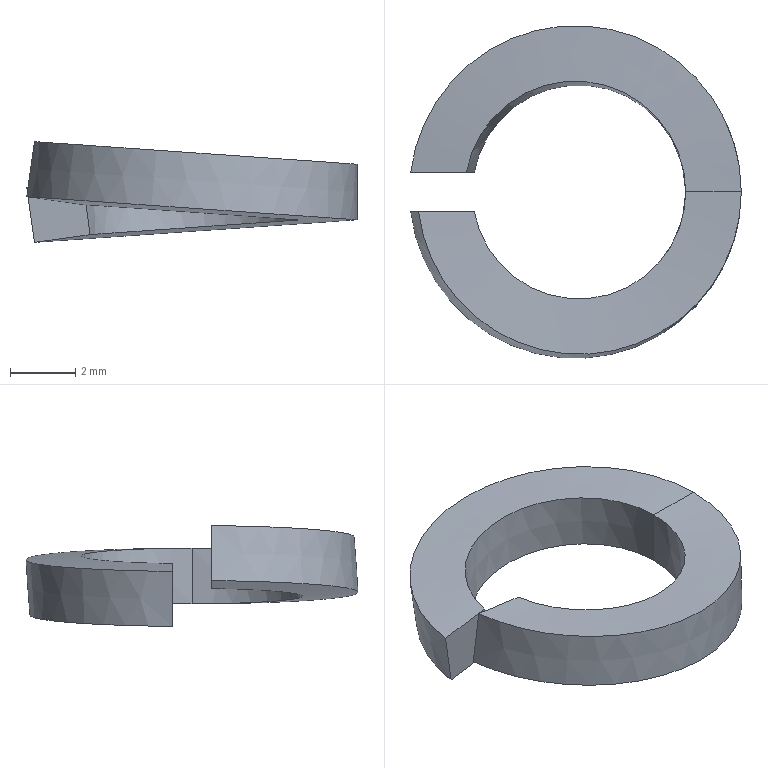Part | NX | features BREP 1 | 1 solid | 10 faces | box 10.114 x 10.174 x 3.081 mm | volume 72.418 mm3 | cone 8 | plane 2
STEP:
#1=CARTESIAN_POINT('',(-3.134,-0.6,2.153));
#2=VERTEX_POINT('',#1);
#3=CARTESIAN_POINT('',(-3.372,-0.6,0.4694));
#4=VERTEX_POINT('',#3);
#5=CARTESIAN_POINT('',(-3.134,-0.6,2.153));
#6=CARTESIAN_POINT('',(-3.169,-0.6,1.904));
#7=CARTESIAN_POINT('',(-3.204,-0.6,1.655));
#8=CARTESIAN_POINT('',(-3.278,-0.6,1.134));
#9=CARTESIAN_POINT('',(-3.317,-0.6,0.8621));
#10=CARTESIAN_POINT('',(-3.361,-0.6,0.5497));
#11=CARTESIAN_POINT('',(-3.367,-0.6,0.5096));
#12=CARTESIAN_POINT('',(-3.372,-0.6,0.4694));
#13=B_SPLINE_CURVE_WITH_KNOTS('',3,(#5,#6,#7,#8,#9,#10,#11,#12),.UNSPECIFIED.,.F.,.F.,(4,2,2,4),(0.,0.4433,0.9284,1.),.UNSPECIFIED.);
#14=EDGE_CURVE('',#2,#4,#13,.T.);
#15=ORIENTED_EDGE('',*,*,#14,.F.);
#16=CARTESIAN_POINT('',(3.34,0.,1.7));
#17=VERTEX_POINT('',#16);
#18=CARTESIAN_POINT('',(0.0754,0.,1.928));
#19=DIRECTION('',(0.06976,0.,0.9976));
#20=DIRECTION('',(0.9976,0.,-0.06976));
#21=AXIS2_PLACEMENT_3D('',#18,#19,#20);
#22=CIRCLE('',#21,3.273);
#23=EDGE_CURVE('',#2,#17,#22,.T.);
#24=ORIENTED_EDGE('',*,*,#23,.T.);
#25=CARTESIAN_POINT('',(3.34,0.,0.));
#26=VERTEX_POINT('',#25);
#27=CARTESIAN_POINT('',(3.34,0.,0.));
#28=DIRECTION('',(0.,0.,1.));
#29=VECTOR('',#28,1000.);
#30=LINE('',#27,#29);
#31=EDGE_CURVE('',#26,#17,#30,.T.);
#32=ORIENTED_EDGE('',*,*,#31,.F.);
#33=CARTESIAN_POINT('',(-0.0429,0.,0.2366));
#34=DIRECTION('',(0.06976,0.,0.9976));
#35=DIRECTION('',(0.9976,0.,-0.06976));
#36=AXIS2_PLACEMENT_3D('',#33,#34,#35);
#37=CIRCLE('',#36,3.391);
#38=EDGE_CURVE('',#4,#26,#37,.T.);
#39=ORIENTED_EDGE('',*,*,#38,.F.);
#40=EDGE_LOOP('',(#15,#24,#32,#39));
#41=FACE_BOUND('',#40,.T.);
#42=CARTESIAN_POINT('',(-0.0429,0.,0.2366));
#43=DIRECTION('',(-0.06976,0.,-0.9976));
#44=DIRECTION('',(0.9976,0.,-0.06976));
#45=AXIS2_PLACEMENT_3D('',#42,#43,#44);
#46=CONICAL_SURFACE('',#45,3.391,0.06981);
#47=ADVANCED_FACE('',(#41),#46,.F.);
#48=CARTESIAN_POINT('',(-4.836,-0.6,2.391));
#49=VERTEX_POINT('',#48);
#50=CARTESIAN_POINT('',(-4.836,-0.6,2.391));
#51=CARTESIAN_POINT('',(-4.269,-0.6,2.311));
#52=CARTESIAN_POINT('',(-3.701,-0.6,2.232));
#53=CARTESIAN_POINT('',(-3.134,-0.6,2.153));
#54=B_SPLINE_CURVE_WITH_KNOTS('',3,(#50,#51,#52,#53),.UNSPECIFIED.,.F.,.F.,(4,4),(0.,1.),.PIECEWISE_BEZIER_KNOTS.);
#55=EDGE_CURVE('',#49,#2,#54,.T.);
#56=ORIENTED_EDGE('',*,*,#55,.F.);
#57=CARTESIAN_POINT('',(5.04,0.,1.7));
#58=VERTEX_POINT('',#57);
#59=CARTESIAN_POINT('',(0.08367,0.,2.047));
#60=DIRECTION('',(0.06976,0.,0.9976));
#61=DIRECTION('',(0.9976,0.,-0.06976));
#62=AXIS2_PLACEMENT_3D('',#59,#60,#61);
#63=CIRCLE('',#62,4.968);
#64=EDGE_CURVE('',#49,#58,#63,.T.);
#65=ORIENTED_EDGE('',*,*,#64,.T.);
#66=CARTESIAN_POINT('',(3.34,0.,1.7));
#67=DIRECTION('',(1.,0.,0.));
#68=VECTOR('',#67,1000.);
#69=LINE('',#66,#68);
#70=EDGE_CURVE('',#17,#58,#69,.T.);
#71=ORIENTED_EDGE('',*,*,#70,.F.);
#72=ORIENTED_EDGE('',*,*,#23,.F.);
#73=EDGE_LOOP('',(#56,#65,#71,#72));
#74=FACE_BOUND('',#73,.T.);
#75=CARTESIAN_POINT('',(0.0754,0.,1.928));
#76=DIRECTION('',(0.06976,0.,0.9976));
#77=DIRECTION('',(-0.9976,0.,0.06976));
#78=AXIS2_PLACEMENT_3D('',#75,#76,#77);
#79=CONICAL_SURFACE('',#78,3.273,1.501);
#80=ADVANCED_FACE('',(#74),#79,.F.);
#81=CARTESIAN_POINT('',(-5.074,-0.6,0.7072));
#82=VERTEX_POINT('',#81);
#83=CARTESIAN_POINT('',(-5.074,-0.6,0.7072));
#84=CARTESIAN_POINT('',(-4.995,-0.6,1.268));
#85=CARTESIAN_POINT('',(-4.916,-0.6,1.829));
#86=CARTESIAN_POINT('',(-4.836,-0.6,2.391));
#87=B_SPLINE_CURVE_WITH_KNOTS('',3,(#83,#84,#85,#86),.UNSPECIFIED.,.F.,.F.,(4,4),(0.,1.),.PIECEWISE_BEZIER_KNOTS.);
#88=EDGE_CURVE('',#82,#49,#87,.T.);
#89=ORIENTED_EDGE('',*,*,#88,.F.);
#90=CARTESIAN_POINT('',(5.04,0.,0.));
#91=VERTEX_POINT('',#90);
#92=CARTESIAN_POINT('',(-0.03462,0.,0.3549));
#93=DIRECTION('',(0.06976,0.,0.9976));
#94=DIRECTION('',(0.9976,0.,-0.06976));
#95=AXIS2_PLACEMENT_3D('',#92,#93,#94);
#96=CIRCLE('',#95,5.087);
#97=EDGE_CURVE('',#82,#91,#96,.T.);
#98=ORIENTED_EDGE('',*,*,#97,.T.);
#99=CARTESIAN_POINT('',(5.04,0.,1.7));
#100=DIRECTION('',(0.,0.,-1.));
#101=VECTOR('',#100,1000.);
#102=LINE('',#99,#101);
#103=EDGE_CURVE('',#58,#91,#102,.T.);
#104=ORIENTED_EDGE('',*,*,#103,.F.);
#105=ORIENTED_EDGE('',*,*,#64,.F.);
#106=EDGE_LOOP('',(#89,#98,#104,#105));
#107=FACE_BOUND('',#106,.T.);
#108=CARTESIAN_POINT('',(0.08367,0.,2.047));
#109=DIRECTION('',(-0.06976,0.,-0.9976));
#110=DIRECTION('',(0.9976,0.,-0.06976));
#111=AXIS2_PLACEMENT_3D('',#108,#109,#110);
#112=CONICAL_SURFACE('',#111,4.968,0.06981);
#113=ADVANCED_FACE('',(#107),#112,.T.);
#114=CARTESIAN_POINT('',(-3.372,-0.6,0.4694));
#115=CARTESIAN_POINT('',(-3.94,-0.6,0.5485));
#116=CARTESIAN_POINT('',(-4.507,-0.6,0.6278));
#117=CARTESIAN_POINT('',(-5.074,-0.6,0.7072));
#118=B_SPLINE_CURVE_WITH_KNOTS('',3,(#114,#115,#116,#117),.UNSPECIFIED.,.F.,.F.,(4,4),(0.,1.),.PIECEWISE_BEZIER_KNOTS.);
#119=EDGE_CURVE('',#4,#82,#118,.T.);
#120=ORIENTED_EDGE('',*,*,#119,.F.);
#121=ORIENTED_EDGE('',*,*,#38,.T.);
#122=CARTESIAN_POINT('',(5.04,0.,0.));
#123=DIRECTION('',(-1.,0.,0.));
#124=VECTOR('',#123,1000.);
#125=LINE('',#122,#124);
#126=EDGE_CURVE('',#91,#26,#125,.T.);
#127=ORIENTED_EDGE('',*,*,#126,.F.);
#128=ORIENTED_EDGE('',*,*,#97,.F.);
#129=EDGE_LOOP('',(#120,#121,#127,#128));
#130=FACE_BOUND('',#129,.T.);
#131=CARTESIAN_POINT('',(-0.03462,0.,0.3549));
#132=DIRECTION('',(0.06976,0.,0.9976));
#133=DIRECTION('',(-0.9976,0.,0.06976));
#134=AXIS2_PLACEMENT_3D('',#131,#132,#133);
#135=CONICAL_SURFACE('',#134,5.087,1.501);
#136=ADVANCED_FACE('',(#130),#135,.T.);
#137=CARTESIAN_POINT('',(-3.372,0.6,1.231));
#138=VERTEX_POINT('',#137);
#139=CARTESIAN_POINT('',(-0.0429,0.,1.463));
#140=DIRECTION('',(0.06976,0.,-0.9976));
#141=DIRECTION('',(-0.9976,0.,-0.06976));
#142=AXIS2_PLACEMENT_3D('',#139,#140,#141);
#143=CIRCLE('',#142,3.391);
#144=EDGE_CURVE('',#138,#17,#143,.T.);
#145=ORIENTED_EDGE('',*,*,#144,.F.);
#146=CARTESIAN_POINT('',(-3.134,0.6,-0.4527));
#147=VERTEX_POINT('',#146);
#148=CARTESIAN_POINT('',(-3.372,0.6,1.231));
#149=CARTESIAN_POINT('',(-3.317,0.6,0.8381));
#150=CARTESIAN_POINT('',(-3.261,0.6,0.4456));
#151=CARTESIAN_POINT('',(-3.182,0.6,-0.1155));
#152=CARTESIAN_POINT('',(-3.158,0.6,-0.2841));
#153=CARTESIAN_POINT('',(-3.134,0.6,-0.4527));
#154=B_SPLINE_CURVE_WITH_KNOTS('',3,(#148,#149,#150,#151,#152,#153),.UNSPECIFIED.,.F.,.F.,(4,2,4),(0.,0.6995,1.),.UNSPECIFIED.);
#155=EDGE_CURVE('',#138,#147,#154,.T.);
#156=ORIENTED_EDGE('',*,*,#155,.T.);
#157=CARTESIAN_POINT('',(0.0754,0.,-0.2283));
#158=DIRECTION('',(0.06976,0.,-0.9976));
#159=DIRECTION('',(-0.9976,0.,-0.06976));
#160=AXIS2_PLACEMENT_3D('',#157,#158,#159);
#161=CIRCLE('',#160,3.273);
#162=EDGE_CURVE('',#147,#26,#161,.T.);
#163=ORIENTED_EDGE('',*,*,#162,.T.);
#164=ORIENTED_EDGE('',*,*,#31,.T.);
#165=EDGE_LOOP('',(#145,#156,#163,#164));
#166=FACE_BOUND('',#165,.T.);
#167=CARTESIAN_POINT('',(0.0754,0.,-0.2283));
#168=DIRECTION('',(-0.06976,0.,0.9976));
#169=DIRECTION('',(-0.9976,0.,-0.06976));
#170=AXIS2_PLACEMENT_3D('',#167,#168,#169);
#171=CONICAL_SURFACE('',#170,3.273,0.06981);
#172=ADVANCED_FACE('',(#166),#171,.F.);
#173=CARTESIAN_POINT('',(-5.074,0.6,0.9928));
#174=VERTEX_POINT('',#173);
#175=CARTESIAN_POINT('',(-0.03462,0.,1.345));
#176=DIRECTION('',(0.06976,0.,-0.9976));
#177=DIRECTION('',(-0.9976,0.,-0.06976));
#178=AXIS2_PLACEMENT_3D('',#175,#176,#177);
#179=CIRCLE('',#178,5.087);
#180=EDGE_CURVE('',#174,#58,#179,.T.);
#181=ORIENTED_EDGE('',*,*,#180,.F.);
#182=CARTESIAN_POINT('',(-5.074,0.6,0.9928));
#183=CARTESIAN_POINT('',(-4.507,0.6,1.072));
#184=CARTESIAN_POINT('',(-3.94,0.6,1.152));
#185=CARTESIAN_POINT('',(-3.372,0.6,1.231));
#186=B_SPLINE_CURVE_WITH_KNOTS('',3,(#182,#183,#184,#185),.UNSPECIFIED.,.F.,.F.,(4,4),(0.,1.),.PIECEWISE_BEZIER_KNOTS.);
#187=EDGE_CURVE('',#174,#138,#186,.T.);
#188=ORIENTED_EDGE('',*,*,#187,.T.);
#189=ORIENTED_EDGE('',*,*,#144,.T.);
#190=ORIENTED_EDGE('',*,*,#70,.T.);
#191=EDGE_LOOP('',(#181,#188,#189,#190));
#192=FACE_BOUND('',#191,.T.);
#193=CARTESIAN_POINT('',(-0.0429,0.,1.463));
#194=DIRECTION('',(0.06976,0.,-0.9976));
#195=DIRECTION('',(0.9976,0.,0.06976));
#196=AXIS2_PLACEMENT_3D('',#193,#194,#195);
#197=CONICAL_SURFACE('',#196,3.391,1.501);
#198=ADVANCED_FACE('',(#192),#197,.T.);
#199=CARTESIAN_POINT('',(-4.836,0.6,-0.6906));
#200=VERTEX_POINT('',#199);
#201=CARTESIAN_POINT('',(0.08367,0.,-0.3466));
#202=DIRECTION('',(0.06976,0.,-0.9976));
#203=DIRECTION('',(-0.9976,0.,-0.06976));
#204=AXIS2_PLACEMENT_3D('',#201,#202,#203);
#205=CIRCLE('',#204,4.968);
#206=EDGE_CURVE('',#200,#91,#205,.T.);
#207=ORIENTED_EDGE('',*,*,#206,.F.);
#208=CARTESIAN_POINT('',(-4.836,0.6,-0.6906));
#209=CARTESIAN_POINT('',(-4.861,0.6,-0.5128));
#210=CARTESIAN_POINT('',(-4.887,0.6,-0.335));
#211=CARTESIAN_POINT('',(-4.966,0.6,0.2262));
#212=CARTESIAN_POINT('',(-5.02,0.6,0.6095));
#213=CARTESIAN_POINT('',(-5.074,0.6,0.9928));
#214=B_SPLINE_CURVE_WITH_KNOTS('',3,(#208,#209,#210,#211,#212,#213),.UNSPECIFIED.,.F.,.F.,(4,2,4),(0.,0.3169,1.),.UNSPECIFIED.);
#215=EDGE_CURVE('',#200,#174,#214,.T.);
#216=ORIENTED_EDGE('',*,*,#215,.T.);
#217=ORIENTED_EDGE('',*,*,#180,.T.);
#218=ORIENTED_EDGE('',*,*,#103,.T.);
#219=EDGE_LOOP('',(#207,#216,#217,#218));
#220=FACE_BOUND('',#219,.T.);
#221=CARTESIAN_POINT('',(-0.03462,0.,1.345));
#222=DIRECTION('',(-0.06976,0.,0.9976));
#223=DIRECTION('',(-0.9976,0.,-0.06976));
#224=AXIS2_PLACEMENT_3D('',#221,#222,#223);
#225=CONICAL_SURFACE('',#224,5.087,0.06981);
#226=ADVANCED_FACE('',(#220),#225,.T.);
#227=ORIENTED_EDGE('',*,*,#162,.F.);
#228=CARTESIAN_POINT('',(-3.134,0.6,-0.4527));
#229=CARTESIAN_POINT('',(-3.701,0.6,-0.5318));
#230=CARTESIAN_POINT('',(-4.269,0.6,-0.6112));
#231=CARTESIAN_POINT('',(-4.836,0.6,-0.6906));
#232=B_SPLINE_CURVE_WITH_KNOTS('',3,(#228,#229,#230,#231),.UNSPECIFIED.,.F.,.F.,(4,4),(0.,1.),.PIECEWISE_BEZIER_KNOTS.);
#233=EDGE_CURVE('',#147,#200,#232,.T.);
#234=ORIENTED_EDGE('',*,*,#233,.T.);
#235=ORIENTED_EDGE('',*,*,#206,.T.);
#236=ORIENTED_EDGE('',*,*,#126,.T.);
#237=EDGE_LOOP('',(#227,#234,#235,#236));
#238=FACE_BOUND('',#237,.T.);
#239=CARTESIAN_POINT('',(0.08367,0.,-0.3466));
#240=DIRECTION('',(0.06976,0.,-0.9976));
#241=DIRECTION('',(0.9976,0.,0.06976));
#242=AXIS2_PLACEMENT_3D('',#239,#240,#241);
#243=CONICAL_SURFACE('',#242,4.968,1.501);
#244=ADVANCED_FACE('',(#238),#243,.F.);
#245=ORIENTED_EDGE('',*,*,#187,.F.);
#246=ORIENTED_EDGE('',*,*,#215,.F.);
#247=ORIENTED_EDGE('',*,*,#233,.F.);
#248=ORIENTED_EDGE('',*,*,#155,.F.);
#249=EDGE_LOOP('',(#245,#246,#247,#248));
#250=FACE_BOUND('',#249,.T.);
#251=CARTESIAN_POINT('',(0.,0.6,-10.08));
#252=DIRECTION('',(0.,1.,0.));
#253=DIRECTION('',(0.,0.,-1.));
#254=AXIS2_PLACEMENT_3D('',#251,#252,#253);
#255=PLANE('',#254);
#256=ADVANCED_FACE('',(#250),#255,.F.);
#257=ORIENTED_EDGE('',*,*,#14,.T.);
#258=ORIENTED_EDGE('',*,*,#119,.T.);
#259=ORIENTED_EDGE('',*,*,#88,.T.);
#260=ORIENTED_EDGE('',*,*,#55,.T.);
#261=EDGE_LOOP('',(#257,#258,#259,#260));
#262=FACE_BOUND('',#261,.T.);
#263=CARTESIAN_POINT('',(-10.08,-0.6,-10.08));
#264=DIRECTION('',(0.,-1.,0.));
#265=DIRECTION('',(0.,0.,1.));
#266=AXIS2_PLACEMENT_3D('',#263,#264,#265);
#267=PLANE('',#266);
#268=ADVANCED_FACE('',(#262),#267,.F.);
#269=CLOSED_SHELL('',(#47,#80,#113,#136,#172,#198,#226,#244,#256,#268));
#270=MANIFOLD_SOLID_BREP('',#269);
#271=(LENGTH_UNIT()NAMED_UNIT(*)SI_UNIT(.MILLI.,.METRE.));
#272=UNCERTAINTY_MEASURE_WITH_UNIT(LENGTH_MEASURE(0.00001),#271,'','');
#273=(NAMED_UNIT(*)PLANE_ANGLE_UNIT()SI_UNIT($,.RADIAN.));
#274=(NAMED_UNIT(*)SI_UNIT($,.STERADIAN.)SOLID_ANGLE_UNIT());
#275=(GEOMETRIC_REPRESENTATION_CONTEXT(3)GLOBAL_UNCERTAINTY_ASSIGNED_CONTEXT((#272))GLOBAL_UNIT_ASSIGNED_CONTEXT((#271,#273,#274))REPRESENTATION_CONTEXT('',''));
#276=ADVANCED_BREP_SHAPE_REPRESENTATION('',(#270),#275);